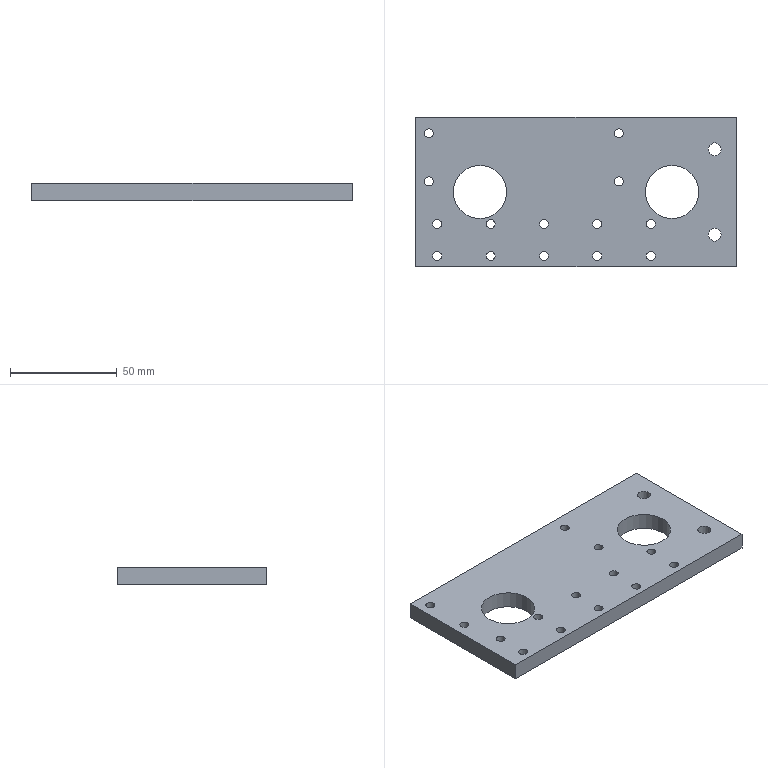Part | NX | 1 solid | 24 faces | box 150 x 70 x 8 mm | volume 74142 mm3 | cylinder 18 | plane 6 | commonest cylinder face diameters 4.2 x14 6 x2 25 x2
STEP:
#1=CARTESIAN_POINT('',(-75.,35.,-4.));
#2=VERTEX_POINT('',#1);
#3=CARTESIAN_POINT('',(-75.,-35.,-4.));
#4=VERTEX_POINT('',#3);
#5=CARTESIAN_POINT('',(-75.,35.,-4.));
#6=DIRECTION('',(0.,-1.,0.));
#7=VECTOR('',#6,1000.);
#8=LINE('',#5,#7);
#9=EDGE_CURVE('',#2,#4,#8,.T.);
#10=ORIENTED_EDGE('',*,*,#9,.T.);
#11=CARTESIAN_POINT('',(-75.,-35.,4.));
#12=VERTEX_POINT('',#11);
#13=CARTESIAN_POINT('',(-75.,-35.,4.));
#14=DIRECTION('',(0.,0.,-1.));
#15=VECTOR('',#14,1000.);
#16=LINE('',#13,#15);
#17=EDGE_CURVE('',#12,#4,#16,.T.);
#18=ORIENTED_EDGE('',*,*,#17,.F.);
#19=CARTESIAN_POINT('',(-75.,35.,4.));
#20=VERTEX_POINT('',#19);
#21=CARTESIAN_POINT('',(-75.,35.,4.));
#22=DIRECTION('',(0.,-1.,0.));
#23=VECTOR('',#22,1000.);
#24=LINE('',#21,#23);
#25=EDGE_CURVE('',#20,#12,#24,.T.);
#26=ORIENTED_EDGE('',*,*,#25,.F.);
#27=CARTESIAN_POINT('',(-75.,35.,4.));
#28=DIRECTION('',(0.,0.,-1.));
#29=VECTOR('',#28,1000.);
#30=LINE('',#27,#29);
#31=EDGE_CURVE('',#20,#2,#30,.T.);
#32=ORIENTED_EDGE('',*,*,#31,.T.);
#33=EDGE_LOOP('',(#10,#18,#26,#32));
#34=FACE_BOUND('',#33,.T.);
#35=CARTESIAN_POINT('',(-75.,35.,4.));
#36=DIRECTION('',(1.,0.,0.));
#37=DIRECTION('',(0.,0.,-1.));
#38=AXIS2_PLACEMENT_3D('',#35,#36,#37);
#39=PLANE('',#38);
#40=ADVANCED_FACE('',(#34),#39,.F.);
#41=CARTESIAN_POINT('',(75.,-35.,-4.));
#42=VERTEX_POINT('',#41);
#43=CARTESIAN_POINT('',(75.,-35.,-4.));
#44=DIRECTION('',(1.,0.,0.));
#45=VECTOR('',#44,1000.);
#46=LINE('',#43,#45);
#47=EDGE_CURVE('',#4,#42,#46,.T.);
#48=ORIENTED_EDGE('',*,*,#47,.T.);
#49=CARTESIAN_POINT('',(75.,-35.,4.));
#50=VERTEX_POINT('',#49);
#51=CARTESIAN_POINT('',(75.,-35.,4.));
#52=DIRECTION('',(0.,0.,-1.));
#53=VECTOR('',#52,1000.);
#54=LINE('',#51,#53);
#55=EDGE_CURVE('',#50,#42,#54,.T.);
#56=ORIENTED_EDGE('',*,*,#55,.F.);
#57=CARTESIAN_POINT('',(75.,-35.,4.));
#58=DIRECTION('',(1.,0.,0.));
#59=VECTOR('',#58,1000.);
#60=LINE('',#57,#59);
#61=EDGE_CURVE('',#12,#50,#60,.T.);
#62=ORIENTED_EDGE('',*,*,#61,.F.);
#63=ORIENTED_EDGE('',*,*,#17,.T.);
#64=EDGE_LOOP('',(#48,#56,#62,#63));
#65=FACE_BOUND('',#64,.T.);
#66=CARTESIAN_POINT('',(75.,-35.,4.));
#67=DIRECTION('',(0.,1.,0.));
#68=DIRECTION('',(-1.,0.,0.));
#69=AXIS2_PLACEMENT_3D('',#66,#67,#68);
#70=PLANE('',#69);
#71=ADVANCED_FACE('',(#65),#70,.F.);
#72=CARTESIAN_POINT('',(75.,35.,-4.));
#73=VERTEX_POINT('',#72);
#74=CARTESIAN_POINT('',(75.,35.,-4.));
#75=DIRECTION('',(0.,1.,0.));
#76=VECTOR('',#75,1000.);
#77=LINE('',#74,#76);
#78=EDGE_CURVE('',#42,#73,#77,.T.);
#79=ORIENTED_EDGE('',*,*,#78,.T.);
#80=CARTESIAN_POINT('',(75.,35.,4.));
#81=VERTEX_POINT('',#80);
#82=CARTESIAN_POINT('',(75.,35.,4.));
#83=DIRECTION('',(0.,0.,-1.));
#84=VECTOR('',#83,1000.);
#85=LINE('',#82,#84);
#86=EDGE_CURVE('',#81,#73,#85,.T.);
#87=ORIENTED_EDGE('',*,*,#86,.F.);
#88=CARTESIAN_POINT('',(75.,35.,4.));
#89=DIRECTION('',(0.,1.,0.));
#90=VECTOR('',#89,1000.);
#91=LINE('',#88,#90);
#92=EDGE_CURVE('',#50,#81,#91,.T.);
#93=ORIENTED_EDGE('',*,*,#92,.F.);
#94=ORIENTED_EDGE('',*,*,#55,.T.);
#95=EDGE_LOOP('',(#79,#87,#93,#94));
#96=FACE_BOUND('',#95,.T.);
#97=CARTESIAN_POINT('',(75.,35.,4.));
#98=DIRECTION('',(-1.,0.,0.));
#99=DIRECTION('',(0.,-1.,0.));
#100=AXIS2_PLACEMENT_3D('',#97,#98,#99);
#101=PLANE('',#100);
#102=ADVANCED_FACE('',(#96),#101,.F.);
#103=CARTESIAN_POINT('',(75.,35.,-4.));
#104=DIRECTION('',(-1.,0.,0.));
#105=VECTOR('',#104,1000.);
#106=LINE('',#103,#105);
#107=EDGE_CURVE('',#73,#2,#106,.T.);
#108=ORIENTED_EDGE('',*,*,#107,.T.);
#109=ORIENTED_EDGE('',*,*,#31,.F.);
#110=CARTESIAN_POINT('',(75.,35.,4.));
#111=DIRECTION('',(-1.,0.,0.));
#112=VECTOR('',#111,1000.);
#113=LINE('',#110,#112);
#114=EDGE_CURVE('',#81,#20,#113,.T.);
#115=ORIENTED_EDGE('',*,*,#114,.F.);
#116=ORIENTED_EDGE('',*,*,#86,.T.);
#117=EDGE_LOOP('',(#108,#109,#115,#116));
#118=FACE_BOUND('',#117,.T.);
#119=CARTESIAN_POINT('',(75.,35.,4.));
#120=DIRECTION('',(0.,-1.,0.));
#121=DIRECTION('',(1.,0.,0.));
#122=AXIS2_PLACEMENT_3D('',#119,#120,#121);
#123=PLANE('',#122);
#124=ADVANCED_FACE('',(#118),#123,.F.);
#125=CARTESIAN_POINT('',(-37.9,-30.,4.));
#126=VERTEX_POINT('',#125);
#127=CARTESIAN_POINT('',(-40.,-30.,4.));
#128=DIRECTION('',(0.,0.,1.));
#129=DIRECTION('',(1.,0.,0.));
#130=AXIS2_PLACEMENT_3D('',#127,#128,#129);
#131=CIRCLE('',#130,2.1);
#132=EDGE_CURVE('',#126,#126,#131,.T.);
#133=ORIENTED_EDGE('',*,*,#132,.F.);
#134=EDGE_LOOP('',(#133));
#135=FACE_BOUND('',#134,.T.);
#136=CARTESIAN_POINT('',(-62.9,-30.,4.));
#137=VERTEX_POINT('',#136);
#138=CARTESIAN_POINT('',(-65.,-30.,4.));
#139=DIRECTION('',(0.,0.,1.));
#140=DIRECTION('',(1.,0.,0.));
#141=AXIS2_PLACEMENT_3D('',#138,#139,#140);
#142=CIRCLE('',#141,2.1);
#143=EDGE_CURVE('',#137,#137,#142,.T.);
#144=ORIENTED_EDGE('',*,*,#143,.F.);
#145=EDGE_LOOP('',(#144));
#146=FACE_BOUND('',#145,.T.);
#147=CARTESIAN_POINT('',(62.,20.,4.));
#148=VERTEX_POINT('',#147);
#149=CARTESIAN_POINT('',(65.,20.,4.));
#150=DIRECTION('',(0.,0.,-1.));
#151=DIRECTION('',(-1.,0.,0.));
#152=AXIS2_PLACEMENT_3D('',#149,#150,#151);
#153=CIRCLE('',#152,3.);
#154=EDGE_CURVE('',#148,#148,#153,.T.);
#155=ORIENTED_EDGE('',*,*,#154,.T.);
#156=EDGE_LOOP('',(#155));
#157=FACE_BOUND('',#156,.T.);
#158=CARTESIAN_POINT('',(62.,-20.,4.));
#159=VERTEX_POINT('',#158);
#160=CARTESIAN_POINT('',(65.,-20.,4.));
#161=DIRECTION('',(0.,0.,-1.));
#162=DIRECTION('',(-1.,0.,0.));
#163=AXIS2_PLACEMENT_3D('',#160,#161,#162);
#164=CIRCLE('',#163,3.);
#165=EDGE_CURVE('',#159,#159,#164,.T.);
#166=ORIENTED_EDGE('',*,*,#165,.T.);
#167=EDGE_LOOP('',(#166));
#168=FACE_BOUND('',#167,.T.);
#169=CARTESIAN_POINT('',(32.5,0.,4.));
#170=VERTEX_POINT('',#169);
#171=CARTESIAN_POINT('',(45.,0.,4.));
#172=DIRECTION('',(0.,0.,-1.));
#173=DIRECTION('',(-1.,0.,0.));
#174=AXIS2_PLACEMENT_3D('',#171,#172,#173);
#175=CIRCLE('',#174,12.5);
#176=EDGE_CURVE('',#170,#170,#175,.T.);
#177=ORIENTED_EDGE('',*,*,#176,.T.);
#178=EDGE_LOOP('',(#177));
#179=FACE_BOUND('',#178,.T.);
#180=CARTESIAN_POINT('',(-57.5,0.,4.));
#181=VERTEX_POINT('',#180);
#182=CARTESIAN_POINT('',(-45.,0.,4.));
#183=DIRECTION('',(0.,0.,-1.));
#184=DIRECTION('',(-1.,0.,0.));
#185=AXIS2_PLACEMENT_3D('',#182,#183,#184);
#186=CIRCLE('',#185,12.5);
#187=EDGE_CURVE('',#181,#181,#186,.T.);
#188=ORIENTED_EDGE('',*,*,#187,.T.);
#189=EDGE_LOOP('',(#188));
#190=FACE_BOUND('',#189,.T.);
#191=CARTESIAN_POINT('',(-71.1,27.5,4.));
#192=VERTEX_POINT('',#191);
#193=CARTESIAN_POINT('',(-69.,27.5,4.));
#194=DIRECTION('',(0.,0.,-1.));
#195=DIRECTION('',(-1.,0.,0.));
#196=AXIS2_PLACEMENT_3D('',#193,#194,#195);
#197=CIRCLE('',#196,2.1);
#198=EDGE_CURVE('',#192,#192,#197,.T.);
#199=ORIENTED_EDGE('',*,*,#198,.T.);
#200=EDGE_LOOP('',(#199));
#201=FACE_BOUND('',#200,.T.);
#202=CARTESIAN_POINT('',(17.9,27.5,4.));
#203=VERTEX_POINT('',#202);
#204=CARTESIAN_POINT('',(20.,27.5,4.));
#205=DIRECTION('',(0.,0.,-1.));
#206=DIRECTION('',(-1.,0.,0.));
#207=AXIS2_PLACEMENT_3D('',#204,#205,#206);
#208=CIRCLE('',#207,2.1);
#209=EDGE_CURVE('',#203,#203,#208,.T.);
#210=ORIENTED_EDGE('',*,*,#209,.T.);
#211=EDGE_LOOP('',(#210));
#212=FACE_BOUND('',#211,.T.);
#213=CARTESIAN_POINT('',(17.9,5.,4.));
#214=VERTEX_POINT('',#213);
#215=CARTESIAN_POINT('',(20.,5.,4.));
#216=DIRECTION('',(0.,0.,-1.));
#217=DIRECTION('',(-1.,0.,0.));
#218=AXIS2_PLACEMENT_3D('',#215,#216,#217);
#219=CIRCLE('',#218,2.1);
#220=EDGE_CURVE('',#214,#214,#219,.T.);
#221=ORIENTED_EDGE('',*,*,#220,.T.);
#222=EDGE_LOOP('',(#221));
#223=FACE_BOUND('',#222,.T.);
#224=CARTESIAN_POINT('',(-71.1,5.,4.));
#225=VERTEX_POINT('',#224);
#226=CARTESIAN_POINT('',(-69.,5.,4.));
#227=DIRECTION('',(0.,0.,-1.));
#228=DIRECTION('',(-1.,0.,0.));
#229=AXIS2_PLACEMENT_3D('',#226,#227,#228);
#230=CIRCLE('',#229,2.1);
#231=EDGE_CURVE('',#225,#225,#230,.T.);
#232=ORIENTED_EDGE('',*,*,#231,.T.);
#233=EDGE_LOOP('',(#232));
#234=FACE_BOUND('',#233,.T.);
#235=ORIENTED_EDGE('',*,*,#25,.T.);
#236=ORIENTED_EDGE('',*,*,#61,.T.);
#237=ORIENTED_EDGE('',*,*,#92,.T.);
#238=ORIENTED_EDGE('',*,*,#114,.T.);
#239=EDGE_LOOP('',(#235,#236,#237,#238));
#240=FACE_BOUND('',#239,.T.);
#241=CARTESIAN_POINT('',(-12.9,-30.,4.));
#242=VERTEX_POINT('',#241);
#243=CARTESIAN_POINT('',(-15.,-30.,4.));
#244=DIRECTION('',(0.,0.,1.));
#245=DIRECTION('',(1.,0.,0.));
#246=AXIS2_PLACEMENT_3D('',#243,#244,#245);
#247=CIRCLE('',#246,2.1);
#248=EDGE_CURVE('',#242,#242,#247,.T.);
#249=ORIENTED_EDGE('',*,*,#248,.F.);
#250=EDGE_LOOP('',(#249));
#251=FACE_BOUND('',#250,.T.);
#252=CARTESIAN_POINT('',(12.1,-30.,4.));
#253=VERTEX_POINT('',#252);
#254=CARTESIAN_POINT('',(10.,-30.,4.));
#255=DIRECTION('',(0.,0.,1.));
#256=DIRECTION('',(1.,0.,0.));
#257=AXIS2_PLACEMENT_3D('',#254,#255,#256);
#258=CIRCLE('',#257,2.1);
#259=EDGE_CURVE('',#253,#253,#258,.T.);
#260=ORIENTED_EDGE('',*,*,#259,.F.);
#261=EDGE_LOOP('',(#260));
#262=FACE_BOUND('',#261,.T.);
#263=CARTESIAN_POINT('',(37.1,-30.,4.));
#264=VERTEX_POINT('',#263);
#265=CARTESIAN_POINT('',(35.,-30.,4.));
#266=DIRECTION('',(0.,0.,1.));
#267=DIRECTION('',(1.,0.,0.));
#268=AXIS2_PLACEMENT_3D('',#265,#266,#267);
#269=CIRCLE('',#268,2.1);
#270=EDGE_CURVE('',#264,#264,#269,.T.);
#271=ORIENTED_EDGE('',*,*,#270,.F.);
#272=EDGE_LOOP('',(#271));
#273=FACE_BOUND('',#272,.T.);
#274=CARTESIAN_POINT('',(-62.9,-15.,4.));
#275=VERTEX_POINT('',#274);
#276=CARTESIAN_POINT('',(-65.,-15.,4.));
#277=DIRECTION('',(0.,0.,1.));
#278=DIRECTION('',(1.,0.,0.));
#279=AXIS2_PLACEMENT_3D('',#276,#277,#278);
#280=CIRCLE('',#279,2.1);
#281=EDGE_CURVE('',#275,#275,#280,.T.);
#282=ORIENTED_EDGE('',*,*,#281,.F.);
#283=EDGE_LOOP('',(#282));
#284=FACE_BOUND('',#283,.T.);
#285=CARTESIAN_POINT('',(-37.9,-15.,4.));
#286=VERTEX_POINT('',#285);
#287=CARTESIAN_POINT('',(-40.,-15.,4.));
#288=DIRECTION('',(0.,0.,1.));
#289=DIRECTION('',(1.,0.,0.));
#290=AXIS2_PLACEMENT_3D('',#287,#288,#289);
#291=CIRCLE('',#290,2.1);
#292=EDGE_CURVE('',#286,#286,#291,.T.);
#293=ORIENTED_EDGE('',*,*,#292,.F.);
#294=EDGE_LOOP('',(#293));
#295=FACE_BOUND('',#294,.T.);
#296=CARTESIAN_POINT('',(-12.9,-15.,4.));
#297=VERTEX_POINT('',#296);
#298=CARTESIAN_POINT('',(-15.,-15.,4.));
#299=DIRECTION('',(0.,0.,1.));
#300=DIRECTION('',(1.,0.,0.));
#301=AXIS2_PLACEMENT_3D('',#298,#299,#300);
#302=CIRCLE('',#301,2.1);
#303=EDGE_CURVE('',#297,#297,#302,.T.);
#304=ORIENTED_EDGE('',*,*,#303,.F.);
#305=EDGE_LOOP('',(#304));
#306=FACE_BOUND('',#305,.T.);
#307=CARTESIAN_POINT('',(12.1,-15.,4.));
#308=VERTEX_POINT('',#307);
#309=CARTESIAN_POINT('',(10.,-15.,4.));
#310=DIRECTION('',(0.,0.,1.));
#311=DIRECTION('',(1.,0.,0.));
#312=AXIS2_PLACEMENT_3D('',#309,#310,#311);
#313=CIRCLE('',#312,2.1);
#314=EDGE_CURVE('',#308,#308,#313,.T.);
#315=ORIENTED_EDGE('',*,*,#314,.F.);
#316=EDGE_LOOP('',(#315));
#317=FACE_BOUND('',#316,.T.);
#318=CARTESIAN_POINT('',(37.1,-15.,4.));
#319=VERTEX_POINT('',#318);
#320=CARTESIAN_POINT('',(35.,-15.,4.));
#321=DIRECTION('',(0.,0.,1.));
#322=DIRECTION('',(1.,0.,0.));
#323=AXIS2_PLACEMENT_3D('',#320,#321,#322);
#324=CIRCLE('',#323,2.1);
#325=EDGE_CURVE('',#319,#319,#324,.T.);
#326=ORIENTED_EDGE('',*,*,#325,.F.);
#327=EDGE_LOOP('',(#326));
#328=FACE_BOUND('',#327,.T.);
#329=CARTESIAN_POINT('',(0.,0.,4.));
#330=DIRECTION('',(0.,0.,-1.));
#331=DIRECTION('',(-1.,0.,0.));
#332=AXIS2_PLACEMENT_3D('',#329,#330,#331);
#333=PLANE('',#332);
#334=ADVANCED_FACE('',(#135,#146,#157,#168,#179,#190,#201,#212,#223,#234,#240,#251,#262,#273,#284,#295,#306,#317,#328),#333,.F.);
#335=CARTESIAN_POINT('',(-37.9,-30.,-4.));
#336=VERTEX_POINT('',#335);
#337=CARTESIAN_POINT('',(-40.,-30.,-4.));
#338=DIRECTION('',(0.,0.,1.));
#339=DIRECTION('',(1.,0.,0.));
#340=AXIS2_PLACEMENT_3D('',#337,#338,#339);
#341=CIRCLE('',#340,2.1);
#342=EDGE_CURVE('',#336,#336,#341,.T.);
#343=ORIENTED_EDGE('',*,*,#342,.T.);
#344=EDGE_LOOP('',(#343));
#345=FACE_BOUND('',#344,.T.);
#346=CARTESIAN_POINT('',(-62.9,-30.,-4.));
#347=VERTEX_POINT('',#346);
#348=CARTESIAN_POINT('',(-65.,-30.,-4.));
#349=DIRECTION('',(0.,0.,1.));
#350=DIRECTION('',(1.,0.,0.));
#351=AXIS2_PLACEMENT_3D('',#348,#349,#350);
#352=CIRCLE('',#351,2.1);
#353=EDGE_CURVE('',#347,#347,#352,.T.);
#354=ORIENTED_EDGE('',*,*,#353,.T.);
#355=EDGE_LOOP('',(#354));
#356=FACE_BOUND('',#355,.T.);
#357=CARTESIAN_POINT('',(62.,20.,-4.));
#358=VERTEX_POINT('',#357);
#359=CARTESIAN_POINT('',(65.,20.,-4.));
#360=DIRECTION('',(0.,0.,-1.));
#361=DIRECTION('',(-1.,0.,0.));
#362=AXIS2_PLACEMENT_3D('',#359,#360,#361);
#363=CIRCLE('',#362,3.);
#364=EDGE_CURVE('',#358,#358,#363,.T.);
#365=ORIENTED_EDGE('',*,*,#364,.F.);
#366=EDGE_LOOP('',(#365));
#367=FACE_BOUND('',#366,.T.);
#368=CARTESIAN_POINT('',(62.,-20.,-4.));
#369=VERTEX_POINT('',#368);
#370=CARTESIAN_POINT('',(65.,-20.,-4.));
#371=DIRECTION('',(0.,0.,-1.));
#372=DIRECTION('',(-1.,0.,0.));
#373=AXIS2_PLACEMENT_3D('',#370,#371,#372);
#374=CIRCLE('',#373,3.);
#375=EDGE_CURVE('',#369,#369,#374,.T.);
#376=ORIENTED_EDGE('',*,*,#375,.F.);
#377=EDGE_LOOP('',(#376));
#378=FACE_BOUND('',#377,.T.);
#379=CARTESIAN_POINT('',(32.5,0.,-4.));
#380=VERTEX_POINT('',#379);
#381=CARTESIAN_POINT('',(45.,0.,-4.));
#382=DIRECTION('',(0.,0.,-1.));
#383=DIRECTION('',(-1.,0.,0.));
#384=AXIS2_PLACEMENT_3D('',#381,#382,#383);
#385=CIRCLE('',#384,12.5);
#386=EDGE_CURVE('',#380,#380,#385,.T.);
#387=ORIENTED_EDGE('',*,*,#386,.F.);
#388=EDGE_LOOP('',(#387));
#389=FACE_BOUND('',#388,.T.);
#390=CARTESIAN_POINT('',(-57.5,0.,-4.));
#391=VERTEX_POINT('',#390);
#392=CARTESIAN_POINT('',(-45.,0.,-4.));
#393=DIRECTION('',(0.,0.,-1.));
#394=DIRECTION('',(-1.,0.,0.));
#395=AXIS2_PLACEMENT_3D('',#392,#393,#394);
#396=CIRCLE('',#395,12.5);
#397=EDGE_CURVE('',#391,#391,#396,.T.);
#398=ORIENTED_EDGE('',*,*,#397,.F.);
#399=EDGE_LOOP('',(#398));
#400=FACE_BOUND('',#399,.T.);
#401=CARTESIAN_POINT('',(-71.1,27.5,-4.));
#402=VERTEX_POINT('',#401);
#403=CARTESIAN_POINT('',(-69.,27.5,-4.));
#404=DIRECTION('',(0.,0.,-1.));
#405=DIRECTION('',(-1.,0.,0.));
#406=AXIS2_PLACEMENT_3D('',#403,#404,#405);
#407=CIRCLE('',#406,2.1);
#408=EDGE_CURVE('',#402,#402,#407,.T.);
#409=ORIENTED_EDGE('',*,*,#408,.F.);
#410=EDGE_LOOP('',(#409));
#411=FACE_BOUND('',#410,.T.);
#412=CARTESIAN_POINT('',(17.9,27.5,-4.));
#413=VERTEX_POINT('',#412);
#414=CARTESIAN_POINT('',(20.,27.5,-4.));
#415=DIRECTION('',(0.,0.,-1.));
#416=DIRECTION('',(-1.,0.,0.));
#417=AXIS2_PLACEMENT_3D('',#414,#415,#416);
#418=CIRCLE('',#417,2.1);
#419=EDGE_CURVE('',#413,#413,#418,.T.);
#420=ORIENTED_EDGE('',*,*,#419,.F.);
#421=EDGE_LOOP('',(#420));
#422=FACE_BOUND('',#421,.T.);
#423=CARTESIAN_POINT('',(17.9,5.,-4.));
#424=VERTEX_POINT('',#423);
#425=CARTESIAN_POINT('',(20.,5.,-4.));
#426=DIRECTION('',(0.,0.,-1.));
#427=DIRECTION('',(-1.,0.,0.));
#428=AXIS2_PLACEMENT_3D('',#425,#426,#427);
#429=CIRCLE('',#428,2.1);
#430=EDGE_CURVE('',#424,#424,#429,.T.);
#431=ORIENTED_EDGE('',*,*,#430,.F.);
#432=EDGE_LOOP('',(#431));
#433=FACE_BOUND('',#432,.T.);
#434=CARTESIAN_POINT('',(-71.1,5.,-4.));
#435=VERTEX_POINT('',#434);
#436=CARTESIAN_POINT('',(-69.,5.,-4.));
#437=DIRECTION('',(0.,0.,-1.));
#438=DIRECTION('',(-1.,0.,0.));
#439=AXIS2_PLACEMENT_3D('',#436,#437,#438);
#440=CIRCLE('',#439,2.1);
#441=EDGE_CURVE('',#435,#435,#440,.T.);
#442=ORIENTED_EDGE('',*,*,#441,.F.);
#443=EDGE_LOOP('',(#442));
#444=FACE_BOUND('',#443,.T.);
#445=ORIENTED_EDGE('',*,*,#9,.F.);
#446=ORIENTED_EDGE('',*,*,#107,.F.);
#447=ORIENTED_EDGE('',*,*,#78,.F.);
#448=ORIENTED_EDGE('',*,*,#47,.F.);
#449=EDGE_LOOP('',(#445,#446,#447,#448));
#450=FACE_BOUND('',#449,.T.);
#451=CARTESIAN_POINT('',(-12.9,-30.,-4.));
#452=VERTEX_POINT('',#451);
#453=CARTESIAN_POINT('',(-15.,-30.,-4.));
#454=DIRECTION('',(0.,0.,1.));
#455=DIRECTION('',(1.,0.,0.));
#456=AXIS2_PLACEMENT_3D('',#453,#454,#455);
#457=CIRCLE('',#456,2.1);
#458=EDGE_CURVE('',#452,#452,#457,.T.);
#459=ORIENTED_EDGE('',*,*,#458,.T.);
#460=EDGE_LOOP('',(#459));
#461=FACE_BOUND('',#460,.T.);
#462=CARTESIAN_POINT('',(12.1,-30.,-4.));
#463=VERTEX_POINT('',#462);
#464=CARTESIAN_POINT('',(10.,-30.,-4.));
#465=DIRECTION('',(0.,0.,1.));
#466=DIRECTION('',(1.,0.,0.));
#467=AXIS2_PLACEMENT_3D('',#464,#465,#466);
#468=CIRCLE('',#467,2.1);
#469=EDGE_CURVE('',#463,#463,#468,.T.);
#470=ORIENTED_EDGE('',*,*,#469,.T.);
#471=EDGE_LOOP('',(#470));
#472=FACE_BOUND('',#471,.T.);
#473=CARTESIAN_POINT('',(37.1,-30.,-4.));
#474=VERTEX_POINT('',#473);
#475=CARTESIAN_POINT('',(35.,-30.,-4.));
#476=DIRECTION('',(0.,0.,1.));
#477=DIRECTION('',(1.,0.,0.));
#478=AXIS2_PLACEMENT_3D('',#475,#476,#477);
#479=CIRCLE('',#478,2.1);
#480=EDGE_CURVE('',#474,#474,#479,.T.);
#481=ORIENTED_EDGE('',*,*,#480,.T.);
#482=EDGE_LOOP('',(#481));
#483=FACE_BOUND('',#482,.T.);
#484=CARTESIAN_POINT('',(-62.9,-15.,-4.));
#485=VERTEX_POINT('',#484);
#486=CARTESIAN_POINT('',(-65.,-15.,-4.));
#487=DIRECTION('',(0.,0.,1.));
#488=DIRECTION('',(1.,0.,0.));
#489=AXIS2_PLACEMENT_3D('',#486,#487,#488);
#490=CIRCLE('',#489,2.1);
#491=EDGE_CURVE('',#485,#485,#490,.T.);
#492=ORIENTED_EDGE('',*,*,#491,.T.);
#493=EDGE_LOOP('',(#492));
#494=FACE_BOUND('',#493,.T.);
#495=CARTESIAN_POINT('',(-37.9,-15.,-4.));
#496=VERTEX_POINT('',#495);
#497=CARTESIAN_POINT('',(-40.,-15.,-4.));
#498=DIRECTION('',(0.,0.,1.));
#499=DIRECTION('',(1.,0.,0.));
#500=AXIS2_PLACEMENT_3D('',#497,#498,#499);
#501=CIRCLE('',#500,2.1);
#502=EDGE_CURVE('',#496,#496,#501,.T.);
#503=ORIENTED_EDGE('',*,*,#502,.T.);
#504=EDGE_LOOP('',(#503));
#505=FACE_BOUND('',#504,.T.);
#506=CARTESIAN_POINT('',(-12.9,-15.,-4.));
#507=VERTEX_POINT('',#506);
#508=CARTESIAN_POINT('',(-15.,-15.,-4.));
#509=DIRECTION('',(0.,0.,1.));
#510=DIRECTION('',(1.,0.,0.));
#511=AXIS2_PLACEMENT_3D('',#508,#509,#510);
#512=CIRCLE('',#511,2.1);
#513=EDGE_CURVE('',#507,#507,#512,.T.);
#514=ORIENTED_EDGE('',*,*,#513,.T.);
#515=EDGE_LOOP('',(#514));
#516=FACE_BOUND('',#515,.T.);
#517=CARTESIAN_POINT('',(12.1,-15.,-4.));
#518=VERTEX_POINT('',#517);
#519=CARTESIAN_POINT('',(10.,-15.,-4.));
#520=DIRECTION('',(0.,0.,1.));
#521=DIRECTION('',(1.,0.,0.));
#522=AXIS2_PLACEMENT_3D('',#519,#520,#521);
#523=CIRCLE('',#522,2.1);
#524=EDGE_CURVE('',#518,#518,#523,.T.);
#525=ORIENTED_EDGE('',*,*,#524,.T.);
#526=EDGE_LOOP('',(#525));
#527=FACE_BOUND('',#526,.T.);
#528=CARTESIAN_POINT('',(37.1,-15.,-4.));
#529=VERTEX_POINT('',#528);
#530=CARTESIAN_POINT('',(35.,-15.,-4.));
#531=DIRECTION('',(0.,0.,1.));
#532=DIRECTION('',(1.,0.,0.));
#533=AXIS2_PLACEMENT_3D('',#530,#531,#532);
#534=CIRCLE('',#533,2.1);
#535=EDGE_CURVE('',#529,#529,#534,.T.);
#536=ORIENTED_EDGE('',*,*,#535,.T.);
#537=EDGE_LOOP('',(#536));
#538=FACE_BOUND('',#537,.T.);
#539=CARTESIAN_POINT('',(0.,0.,-4.));
#540=DIRECTION('',(0.,0.,-1.));
#541=DIRECTION('',(-1.,0.,0.));
#542=AXIS2_PLACEMENT_3D('',#539,#540,#541);
#543=PLANE('',#542);
#544=ADVANCED_FACE('',(#345,#356,#367,#378,#389,#400,#411,#422,#433,#444,#450,#461,#472,#483,#494,#505,#516,#527,#538),#543,.T.);
#545=ORIENTED_EDGE('',*,*,#231,.F.);
#546=EDGE_LOOP('',(#545));
#547=FACE_BOUND('',#546,.T.);
#548=ORIENTED_EDGE('',*,*,#441,.T.);
#549=EDGE_LOOP('',(#548));
#550=FACE_BOUND('',#549,.T.);
#551=CARTESIAN_POINT('',(-69.,5.,-4.));
#552=DIRECTION('',(0.,0.,-1.));
#553=DIRECTION('',(-1.,0.,0.));
#554=AXIS2_PLACEMENT_3D('',#551,#552,#553);
#555=CYLINDRICAL_SURFACE('',#554,2.1);
#556=ADVANCED_FACE('',(#547,#550),#555,.F.);
#557=ORIENTED_EDGE('',*,*,#220,.F.);
#558=EDGE_LOOP('',(#557));
#559=FACE_BOUND('',#558,.T.);
#560=ORIENTED_EDGE('',*,*,#430,.T.);
#561=EDGE_LOOP('',(#560));
#562=FACE_BOUND('',#561,.T.);
#563=CARTESIAN_POINT('',(20.,5.,-4.));
#564=DIRECTION('',(0.,0.,-1.));
#565=DIRECTION('',(-1.,0.,0.));
#566=AXIS2_PLACEMENT_3D('',#563,#564,#565);
#567=CYLINDRICAL_SURFACE('',#566,2.1);
#568=ADVANCED_FACE('',(#559,#562),#567,.F.);
#569=ORIENTED_EDGE('',*,*,#209,.F.);
#570=EDGE_LOOP('',(#569));
#571=FACE_BOUND('',#570,.T.);
#572=ORIENTED_EDGE('',*,*,#419,.T.);
#573=EDGE_LOOP('',(#572));
#574=FACE_BOUND('',#573,.T.);
#575=CARTESIAN_POINT('',(20.,27.5,-4.));
#576=DIRECTION('',(0.,0.,-1.));
#577=DIRECTION('',(-1.,0.,0.));
#578=AXIS2_PLACEMENT_3D('',#575,#576,#577);
#579=CYLINDRICAL_SURFACE('',#578,2.1);
#580=ADVANCED_FACE('',(#571,#574),#579,.F.);
#581=ORIENTED_EDGE('',*,*,#198,.F.);
#582=EDGE_LOOP('',(#581));
#583=FACE_BOUND('',#582,.T.);
#584=ORIENTED_EDGE('',*,*,#408,.T.);
#585=EDGE_LOOP('',(#584));
#586=FACE_BOUND('',#585,.T.);
#587=CARTESIAN_POINT('',(-69.,27.5,-4.));
#588=DIRECTION('',(0.,0.,-1.));
#589=DIRECTION('',(-1.,0.,0.));
#590=AXIS2_PLACEMENT_3D('',#587,#588,#589);
#591=CYLINDRICAL_SURFACE('',#590,2.1);
#592=ADVANCED_FACE('',(#583,#586),#591,.F.);
#593=ORIENTED_EDGE('',*,*,#187,.F.);
#594=EDGE_LOOP('',(#593));
#595=FACE_BOUND('',#594,.T.);
#596=ORIENTED_EDGE('',*,*,#397,.T.);
#597=EDGE_LOOP('',(#596));
#598=FACE_BOUND('',#597,.T.);
#599=CARTESIAN_POINT('',(-45.,0.,4.));
#600=DIRECTION('',(0.,0.,-1.));
#601=DIRECTION('',(-1.,0.,0.));
#602=AXIS2_PLACEMENT_3D('',#599,#600,#601);
#603=CYLINDRICAL_SURFACE('',#602,12.5);
#604=ADVANCED_FACE('',(#595,#598),#603,.F.);
#605=ORIENTED_EDGE('',*,*,#176,.F.);
#606=EDGE_LOOP('',(#605));
#607=FACE_BOUND('',#606,.T.);
#608=ORIENTED_EDGE('',*,*,#386,.T.);
#609=EDGE_LOOP('',(#608));
#610=FACE_BOUND('',#609,.T.);
#611=CARTESIAN_POINT('',(45.,0.,4.));
#612=DIRECTION('',(0.,0.,-1.));
#613=DIRECTION('',(-1.,0.,0.));
#614=AXIS2_PLACEMENT_3D('',#611,#612,#613);
#615=CYLINDRICAL_SURFACE('',#614,12.5);
#616=ADVANCED_FACE('',(#607,#610),#615,.F.);
#617=ORIENTED_EDGE('',*,*,#165,.F.);
#618=EDGE_LOOP('',(#617));
#619=FACE_BOUND('',#618,.T.);
#620=ORIENTED_EDGE('',*,*,#375,.T.);
#621=EDGE_LOOP('',(#620));
#622=FACE_BOUND('',#621,.T.);
#623=CARTESIAN_POINT('',(65.,-20.,-4.));
#624=DIRECTION('',(0.,0.,-1.));
#625=DIRECTION('',(-1.,0.,0.));
#626=AXIS2_PLACEMENT_3D('',#623,#624,#625);
#627=CYLINDRICAL_SURFACE('',#626,3.);
#628=ADVANCED_FACE('',(#619,#622),#627,.F.);
#629=ORIENTED_EDGE('',*,*,#154,.F.);
#630=EDGE_LOOP('',(#629));
#631=FACE_BOUND('',#630,.T.);
#632=ORIENTED_EDGE('',*,*,#364,.T.);
#633=EDGE_LOOP('',(#632));
#634=FACE_BOUND('',#633,.T.);
#635=CARTESIAN_POINT('',(65.,20.,-4.));
#636=DIRECTION('',(0.,0.,-1.));
#637=DIRECTION('',(-1.,0.,0.));
#638=AXIS2_PLACEMENT_3D('',#635,#636,#637);
#639=CYLINDRICAL_SURFACE('',#638,3.);
#640=ADVANCED_FACE('',(#631,#634),#639,.F.);
#641=ORIENTED_EDGE('',*,*,#353,.F.);
#642=EDGE_LOOP('',(#641));
#643=FACE_BOUND('',#642,.T.);
#644=ORIENTED_EDGE('',*,*,#143,.T.);
#645=EDGE_LOOP('',(#644));
#646=FACE_BOUND('',#645,.T.);
#647=CARTESIAN_POINT('',(-65.,-30.,4.));
#648=DIRECTION('',(0.,0.,1.));
#649=DIRECTION('',(1.,0.,0.));
#650=AXIS2_PLACEMENT_3D('',#647,#648,#649);
#651=CYLINDRICAL_SURFACE('',#650,2.1);
#652=ADVANCED_FACE('',(#643,#646),#651,.F.);
#653=ORIENTED_EDGE('',*,*,#342,.F.);
#654=EDGE_LOOP('',(#653));
#655=FACE_BOUND('',#654,.T.);
#656=ORIENTED_EDGE('',*,*,#132,.T.);
#657=EDGE_LOOP('',(#656));
#658=FACE_BOUND('',#657,.T.);
#659=CARTESIAN_POINT('',(-40.,-30.,4.));
#660=DIRECTION('',(0.,0.,1.));
#661=DIRECTION('',(1.,0.,0.));
#662=AXIS2_PLACEMENT_3D('',#659,#660,#661);
#663=CYLINDRICAL_SURFACE('',#662,2.1);
#664=ADVANCED_FACE('',(#655,#658),#663,.F.);
#665=ORIENTED_EDGE('',*,*,#458,.F.);
#666=EDGE_LOOP('',(#665));
#667=FACE_BOUND('',#666,.T.);
#668=ORIENTED_EDGE('',*,*,#248,.T.);
#669=EDGE_LOOP('',(#668));
#670=FACE_BOUND('',#669,.T.);
#671=CARTESIAN_POINT('',(-15.,-30.,4.));
#672=DIRECTION('',(0.,0.,1.));
#673=DIRECTION('',(1.,0.,0.));
#674=AXIS2_PLACEMENT_3D('',#671,#672,#673);
#675=CYLINDRICAL_SURFACE('',#674,2.1);
#676=ADVANCED_FACE('',(#667,#670),#675,.F.);
#677=ORIENTED_EDGE('',*,*,#469,.F.);
#678=EDGE_LOOP('',(#677));
#679=FACE_BOUND('',#678,.T.);
#680=ORIENTED_EDGE('',*,*,#259,.T.);
#681=EDGE_LOOP('',(#680));
#682=FACE_BOUND('',#681,.T.);
#683=CARTESIAN_POINT('',(10.,-30.,4.));
#684=DIRECTION('',(0.,0.,1.));
#685=DIRECTION('',(1.,0.,0.));
#686=AXIS2_PLACEMENT_3D('',#683,#684,#685);
#687=CYLINDRICAL_SURFACE('',#686,2.1);
#688=ADVANCED_FACE('',(#679,#682),#687,.F.);
#689=ORIENTED_EDGE('',*,*,#480,.F.);
#690=EDGE_LOOP('',(#689));
#691=FACE_BOUND('',#690,.T.);
#692=ORIENTED_EDGE('',*,*,#270,.T.);
#693=EDGE_LOOP('',(#692));
#694=FACE_BOUND('',#693,.T.);
#695=CARTESIAN_POINT('',(35.,-30.,4.));
#696=DIRECTION('',(0.,0.,1.));
#697=DIRECTION('',(1.,0.,0.));
#698=AXIS2_PLACEMENT_3D('',#695,#696,#697);
#699=CYLINDRICAL_SURFACE('',#698,2.1);
#700=ADVANCED_FACE('',(#691,#694),#699,.F.);
#701=ORIENTED_EDGE('',*,*,#491,.F.);
#702=EDGE_LOOP('',(#701));
#703=FACE_BOUND('',#702,.T.);
#704=ORIENTED_EDGE('',*,*,#281,.T.);
#705=EDGE_LOOP('',(#704));
#706=FACE_BOUND('',#705,.T.);
#707=CARTESIAN_POINT('',(-65.,-15.,4.));
#708=DIRECTION('',(0.,0.,1.));
#709=DIRECTION('',(1.,0.,0.));
#710=AXIS2_PLACEMENT_3D('',#707,#708,#709);
#711=CYLINDRICAL_SURFACE('',#710,2.1);
#712=ADVANCED_FACE('',(#703,#706),#711,.F.);
#713=ORIENTED_EDGE('',*,*,#502,.F.);
#714=EDGE_LOOP('',(#713));
#715=FACE_BOUND('',#714,.T.);
#716=ORIENTED_EDGE('',*,*,#292,.T.);
#717=EDGE_LOOP('',(#716));
#718=FACE_BOUND('',#717,.T.);
#719=CARTESIAN_POINT('',(-40.,-15.,4.));
#720=DIRECTION('',(0.,0.,1.));
#721=DIRECTION('',(1.,0.,0.));
#722=AXIS2_PLACEMENT_3D('',#719,#720,#721);
#723=CYLINDRICAL_SURFACE('',#722,2.1);
#724=ADVANCED_FACE('',(#715,#718),#723,.F.);
#725=ORIENTED_EDGE('',*,*,#513,.F.);
#726=EDGE_LOOP('',(#725));
#727=FACE_BOUND('',#726,.T.);
#728=ORIENTED_EDGE('',*,*,#303,.T.);
#729=EDGE_LOOP('',(#728));
#730=FACE_BOUND('',#729,.T.);
#731=CARTESIAN_POINT('',(-15.,-15.,4.));
#732=DIRECTION('',(0.,0.,1.));
#733=DIRECTION('',(1.,0.,0.));
#734=AXIS2_PLACEMENT_3D('',#731,#732,#733);
#735=CYLINDRICAL_SURFACE('',#734,2.1);
#736=ADVANCED_FACE('',(#727,#730),#735,.F.);
#737=ORIENTED_EDGE('',*,*,#524,.F.);
#738=EDGE_LOOP('',(#737));
#739=FACE_BOUND('',#738,.T.);
#740=ORIENTED_EDGE('',*,*,#314,.T.);
#741=EDGE_LOOP('',(#740));
#742=FACE_BOUND('',#741,.T.);
#743=CARTESIAN_POINT('',(10.,-15.,4.));
#744=DIRECTION('',(0.,0.,1.));
#745=DIRECTION('',(1.,0.,0.));
#746=AXIS2_PLACEMENT_3D('',#743,#744,#745);
#747=CYLINDRICAL_SURFACE('',#746,2.1);
#748=ADVANCED_FACE('',(#739,#742),#747,.F.);
#749=ORIENTED_EDGE('',*,*,#535,.F.);
#750=EDGE_LOOP('',(#749));
#751=FACE_BOUND('',#750,.T.);
#752=ORIENTED_EDGE('',*,*,#325,.T.);
#753=EDGE_LOOP('',(#752));
#754=FACE_BOUND('',#753,.T.);
#755=CARTESIAN_POINT('',(35.,-15.,4.));
#756=DIRECTION('',(0.,0.,1.));
#757=DIRECTION('',(1.,0.,0.));
#758=AXIS2_PLACEMENT_3D('',#755,#756,#757);
#759=CYLINDRICAL_SURFACE('',#758,2.1);
#760=ADVANCED_FACE('',(#751,#754),#759,.F.);
#761=CLOSED_SHELL('',(#40,#71,#102,#124,#334,#544,#556,#568,#580,#592,#604,#616,#628,#640,#652,#664,#676,#688,#700,#712,#724,#736,#748,#760));
#762=MANIFOLD_SOLID_BREP('',#761);
#763=(LENGTH_UNIT()NAMED_UNIT(*)SI_UNIT(.MILLI.,.METRE.));
#764=UNCERTAINTY_MEASURE_WITH_UNIT(LENGTH_MEASURE(0.00001),#763,'','');
#765=(NAMED_UNIT(*)PLANE_ANGLE_UNIT()SI_UNIT($,.RADIAN.));
#766=(NAMED_UNIT(*)SI_UNIT($,.STERADIAN.)SOLID_ANGLE_UNIT());
#767=(GEOMETRIC_REPRESENTATION_CONTEXT(3)GLOBAL_UNCERTAINTY_ASSIGNED_CONTEXT((#764))GLOBAL_UNIT_ASSIGNED_CONTEXT((#763,#765,#766))REPRESENTATION_CONTEXT('',''));
#768=ADVANCED_BREP_SHAPE_REPRESENTATION('',(#762),#767);